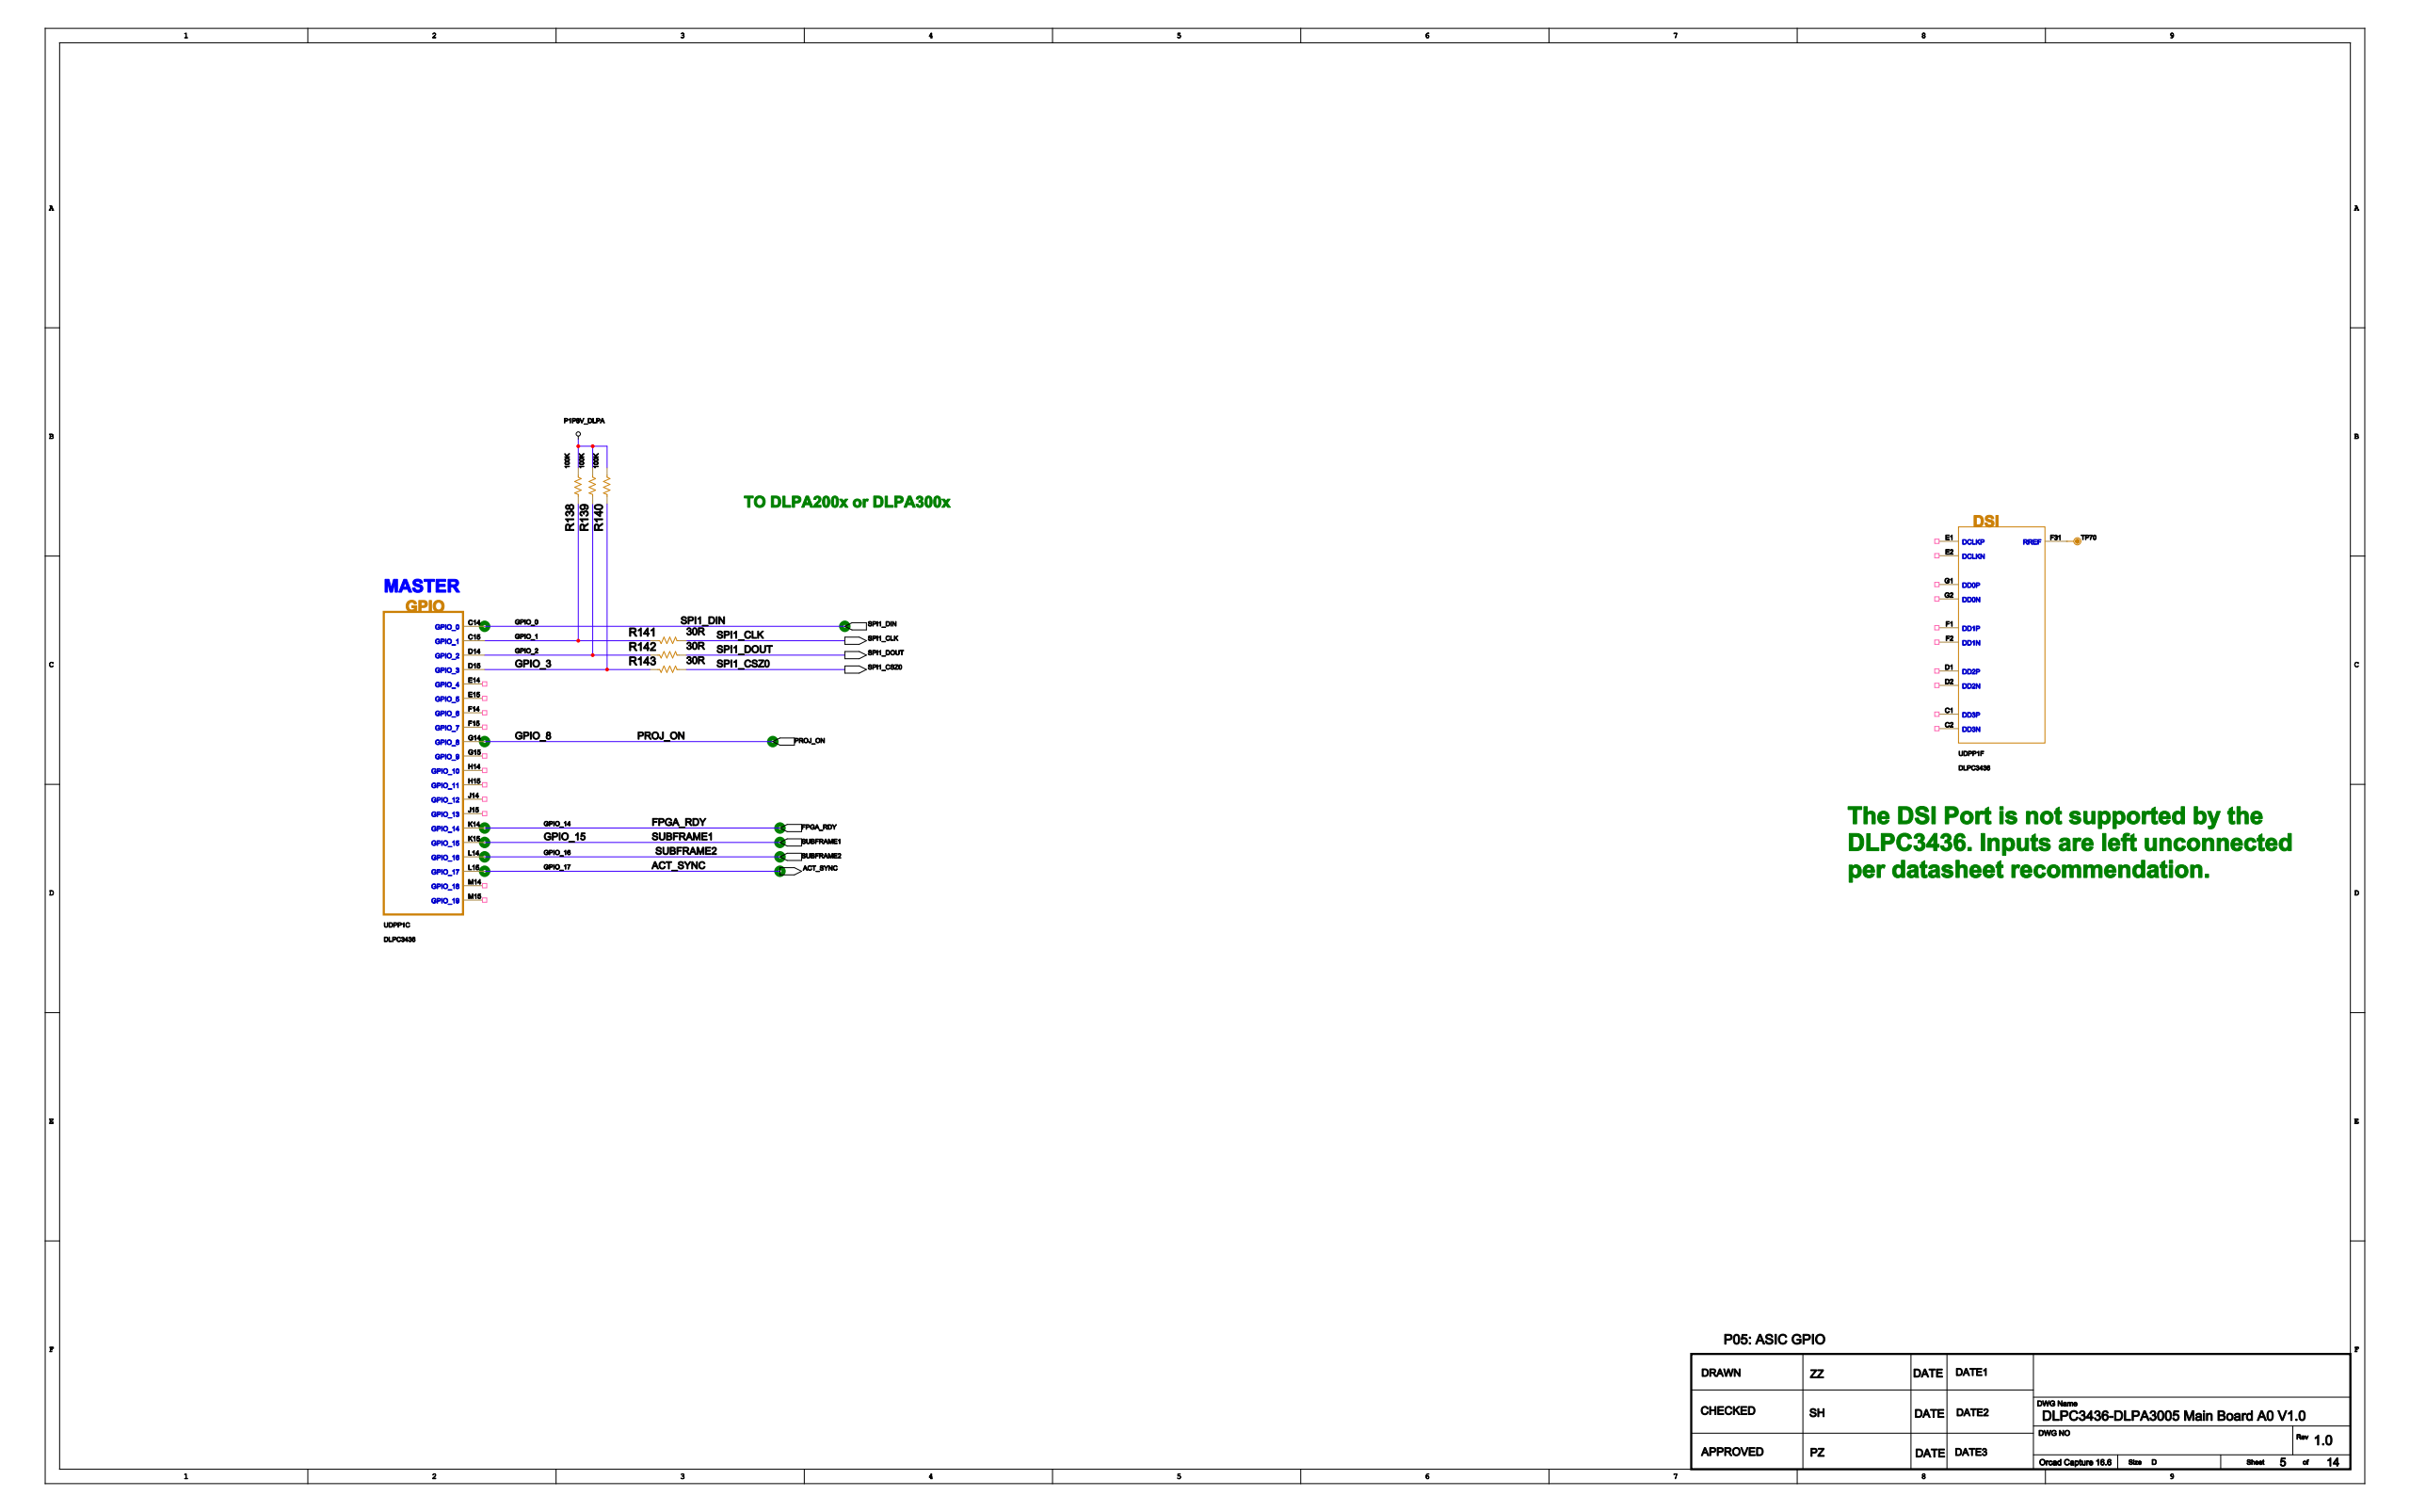Circuit board | Cadence Allegro | 1223 parts | 777 nets | one sheet of the schematic
Parts on this sheet (reference | value | footprint):
R138 | 100K | R0201
R139 | 100K | R0201
R140 | 100K | R0201
R141 | 30R | R0201
R142 | 30R | R0201
R143 | 30R | R0201
TP70 | DEO | TP06MM
UDPP1 | DLPC3436 | DLPC3436_176NFBGA
Nets of these parts (net: part-pin ...):
P1P8V_DLPA: R138-2 R139-2 R140-2
N2554126510: TP70-1 UDPP1-F3
PROJ_ON: UDPP1-G14
GPIO_1: R138-1 R141-2 UDPP1-C15
GPIO_2: R139-1 R142-2 UDPP1-D14
GPIO_3: R140-1 R143-2 UDPP1-D15
SPI1_CLK: R141-1
SPI1_DOUT: R142-1
SPI1_CSZ0: R143-1
SPI1_DIN: UDPP1-C14
FPGA_RDY: UDPP1-K14
ACT_SYNC: UDPP1-L15
SUBFRAME1: UDPP1-K15
SUBFRAME2: UDPP1-L14